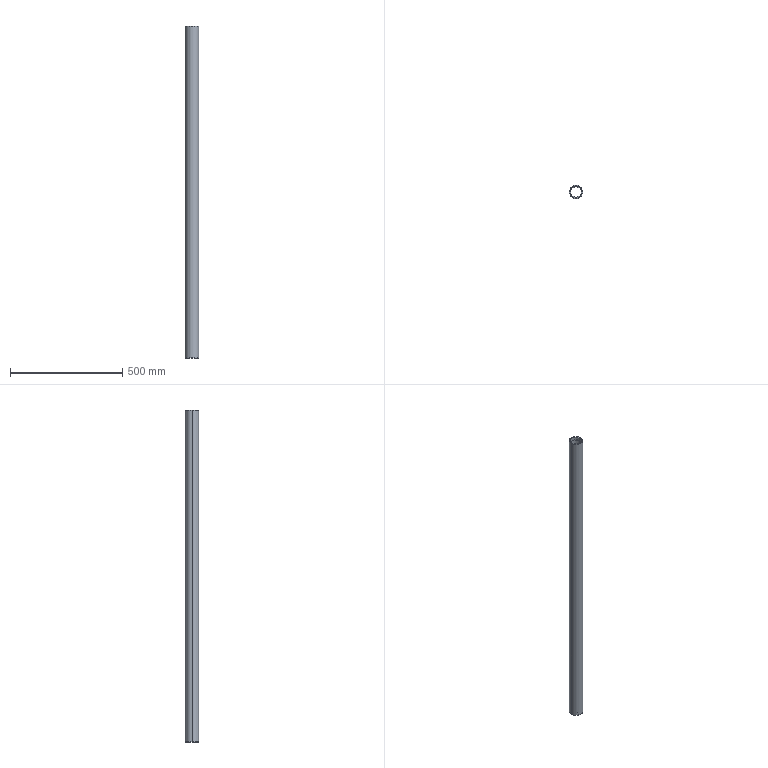Part | SolidWorks | features ICE 3, Chamfer 1, Extrusion 1 | 1 solid | 20 faces | box 60 x 60 x 1480 mm | volume 1496944 mm3 | cone 8 | cylinder 8 | plane 4 | commonest cylinder face diameters 52 x4 48 x2 60 x2
STEP:
#1=CARTESIAN_POINT('',(29.5,0.,1480.));
#2=VERTEX_POINT('',#1);
#3=CARTESIAN_POINT('',(-29.5,0.,1480.));
#4=VERTEX_POINT('',#3);
#5=CARTESIAN_POINT('',(0.,0.,1480.));
#6=DIRECTION('',(0.,0.,1.));
#7=DIRECTION('',(1.,0.,0.));
#8=AXIS2_PLACEMENT_3D('',#5,#6,#7);
#9=CIRCLE('',#8,29.5);
#10=EDGE_CURVE('',#2,#4,#9,.T.);
#11=ORIENTED_EDGE('',*,*,#10,.F.);
#12=CARTESIAN_POINT('',(30.,0.,1479.5));
#13=VERTEX_POINT('',#12);
#14=CARTESIAN_POINT('',(29.5,0.,1480.));
#15=DIRECTION('',(0.7071,0.,-0.7071));
#16=VECTOR('',#15,1000.);
#17=LINE('',#14,#16);
#18=EDGE_CURVE('',#2,#13,#17,.T.);
#19=ORIENTED_EDGE('',*,*,#18,.T.);
#20=CARTESIAN_POINT('',(-30.,0.,1479.5));
#21=VERTEX_POINT('',#20);
#22=CARTESIAN_POINT('',(0.,0.,1479.5));
#23=DIRECTION('',(0.,0.,-1.));
#24=DIRECTION('',(1.,0.,0.));
#25=AXIS2_PLACEMENT_3D('',#22,#23,#24);
#26=CIRCLE('',#25,30.);
#27=EDGE_CURVE('',#21,#13,#26,.T.);
#28=ORIENTED_EDGE('',*,*,#27,.F.);
#29=CARTESIAN_POINT('',(-29.5,0.,1480.));
#30=DIRECTION('',(-0.7071,0.,-0.7071));
#31=VECTOR('',#30,1000.);
#32=LINE('',#29,#31);
#33=EDGE_CURVE('',#4,#21,#32,.T.);
#34=ORIENTED_EDGE('',*,*,#33,.F.);
#35=EDGE_LOOP('',(#11,#19,#28,#34));
#36=FACE_OUTER_BOUND('',#35,.T.);
#37=CARTESIAN_POINT('',(0.,0.,1480.));
#38=DIRECTION('',(0.,0.,-1.));
#39=DIRECTION('',(-1.,0.,0.));
#40=AXIS2_PLACEMENT_3D('',#37,#38,#39);
#41=CONICAL_SURFACE('',#40,29.5,0.7854);
#42=ADVANCED_FACE('',(#36),#41,.T.);
#43=CARTESIAN_POINT('',(-26.,0.,1479.5));
#44=VERTEX_POINT('',#43);
#45=CARTESIAN_POINT('',(26.,0.,1479.5));
#46=VERTEX_POINT('',#45);
#47=CARTESIAN_POINT('',(0.,0.,1479.5));
#48=DIRECTION('',(0.,0.,1.));
#49=DIRECTION('',(1.,0.,0.));
#50=AXIS2_PLACEMENT_3D('',#47,#48,#49);
#51=CIRCLE('',#50,26.);
#52=EDGE_CURVE('',#44,#46,#51,.T.);
#53=ORIENTED_EDGE('',*,*,#52,.F.);
#54=CARTESIAN_POINT('',(-26.5,0.,1480.));
#55=VERTEX_POINT('',#54);
#56=CARTESIAN_POINT('',(-26.,0.,1479.5));
#57=DIRECTION('',(-0.7071,0.,0.7071));
#58=VECTOR('',#57,1000.);
#59=LINE('',#56,#58);
#60=EDGE_CURVE('',#44,#55,#59,.T.);
#61=ORIENTED_EDGE('',*,*,#60,.T.);
#62=CARTESIAN_POINT('',(26.5,0.,1480.));
#63=VERTEX_POINT('',#62);
#64=CARTESIAN_POINT('',(0.,0.,1480.));
#65=DIRECTION('',(0.,0.,-1.));
#66=DIRECTION('',(1.,0.,0.));
#67=AXIS2_PLACEMENT_3D('',#64,#65,#66);
#68=CIRCLE('',#67,26.5);
#69=EDGE_CURVE('',#63,#55,#68,.T.);
#70=ORIENTED_EDGE('',*,*,#69,.F.);
#71=CARTESIAN_POINT('',(26.,0.,1479.5));
#72=DIRECTION('',(0.7071,0.,0.7071));
#73=VECTOR('',#72,1000.);
#74=LINE('',#71,#73);
#75=EDGE_CURVE('',#46,#63,#74,.T.);
#76=ORIENTED_EDGE('',*,*,#75,.F.);
#77=EDGE_LOOP('',(#53,#61,#70,#76));
#78=FACE_OUTER_BOUND('',#77,.T.);
#79=CARTESIAN_POINT('',(0.,0.,1479.5));
#80=DIRECTION('',(0.,0.,1.));
#81=DIRECTION('',(1.,0.,0.));
#82=AXIS2_PLACEMENT_3D('',#79,#80,#81);
#83=CONICAL_SURFACE('',#82,26.,0.7854);
#84=ADVANCED_FACE('',(#78),#83,.F.);
#85=CARTESIAN_POINT('',(-29.5,0.,0.));
#86=VERTEX_POINT('',#85);
#87=CARTESIAN_POINT('',(29.5,0.,0.));
#88=VERTEX_POINT('',#87);
#89=CARTESIAN_POINT('',(0.,0.,0.));
#90=DIRECTION('',(0.,0.,-1.));
#91=DIRECTION('',(1.,0.,0.));
#92=AXIS2_PLACEMENT_3D('',#89,#90,#91);
#93=CIRCLE('',#92,29.5);
#94=EDGE_CURVE('',#86,#88,#93,.T.);
#95=ORIENTED_EDGE('',*,*,#94,.F.);
#96=CARTESIAN_POINT('',(-30.,0.,0.5));
#97=VERTEX_POINT('',#96);
#98=CARTESIAN_POINT('',(-30.,0.,0.5));
#99=DIRECTION('',(-0.7071,0.,0.7071));
#100=VECTOR('',#99,1000.);
#101=LINE('',#98,#100);
#102=EDGE_CURVE('',#86,#97,#101,.T.);
#103=ORIENTED_EDGE('',*,*,#102,.T.);
#104=CARTESIAN_POINT('',(30.,0.,0.5));
#105=VERTEX_POINT('',#104);
#106=CARTESIAN_POINT('',(0.,0.,0.5));
#107=DIRECTION('',(0.,0.,1.));
#108=DIRECTION('',(1.,0.,0.));
#109=AXIS2_PLACEMENT_3D('',#106,#107,#108);
#110=CIRCLE('',#109,30.);
#111=EDGE_CURVE('',#105,#97,#110,.T.);
#112=ORIENTED_EDGE('',*,*,#111,.F.);
#113=CARTESIAN_POINT('',(30.,0.,0.5));
#114=DIRECTION('',(0.7071,0.,0.7071));
#115=VECTOR('',#114,1000.);
#116=LINE('',#113,#115);
#117=EDGE_CURVE('',#88,#105,#116,.T.);
#118=ORIENTED_EDGE('',*,*,#117,.F.);
#119=EDGE_LOOP('',(#95,#103,#112,#118));
#120=FACE_OUTER_BOUND('',#119,.T.);
#121=CARTESIAN_POINT('',(0.,0.,0.5));
#122=DIRECTION('',(0.,0.,1.));
#123=DIRECTION('',(1.,0.,0.));
#124=AXIS2_PLACEMENT_3D('',#121,#122,#123);
#125=CONICAL_SURFACE('',#124,30.,0.7854);
#126=ADVANCED_FACE('',(#120),#125,.T.);
#127=CARTESIAN_POINT('',(26.,0.,0.5));
#128=VERTEX_POINT('',#127);
#129=CARTESIAN_POINT('',(-26.,0.,0.5));
#130=VERTEX_POINT('',#129);
#131=CARTESIAN_POINT('',(0.,0.,0.5));
#132=DIRECTION('',(0.,0.,-1.));
#133=DIRECTION('',(1.,0.,0.));
#134=AXIS2_PLACEMENT_3D('',#131,#132,#133);
#135=CIRCLE('',#134,26.);
#136=EDGE_CURVE('',#128,#130,#135,.T.);
#137=ORIENTED_EDGE('',*,*,#136,.F.);
#138=CARTESIAN_POINT('',(26.5,0.,0.));
#139=VERTEX_POINT('',#138);
#140=CARTESIAN_POINT('',(26.,0.,0.5));
#141=DIRECTION('',(0.7071,0.,-0.7071));
#142=VECTOR('',#141,1000.);
#143=LINE('',#140,#142);
#144=EDGE_CURVE('',#128,#139,#143,.T.);
#145=ORIENTED_EDGE('',*,*,#144,.T.);
#146=CARTESIAN_POINT('',(-26.5,0.,0.));
#147=VERTEX_POINT('',#146);
#148=CARTESIAN_POINT('',(0.,0.,0.));
#149=DIRECTION('',(0.,0.,1.));
#150=DIRECTION('',(1.,0.,0.));
#151=AXIS2_PLACEMENT_3D('',#148,#149,#150);
#152=CIRCLE('',#151,26.5);
#153=EDGE_CURVE('',#147,#139,#152,.T.);
#154=ORIENTED_EDGE('',*,*,#153,.F.);
#155=CARTESIAN_POINT('',(-26.,0.,0.5));
#156=DIRECTION('',(-0.7071,0.,-0.7071));
#157=VECTOR('',#156,1000.);
#158=LINE('',#155,#157);
#159=EDGE_CURVE('',#130,#147,#158,.T.);
#160=ORIENTED_EDGE('',*,*,#159,.F.);
#161=EDGE_LOOP('',(#137,#145,#154,#160));
#162=FACE_OUTER_BOUND('',#161,.T.);
#163=CARTESIAN_POINT('',(0.,0.,0.5));
#164=DIRECTION('',(0.,0.,-1.));
#165=DIRECTION('',(-1.,0.,0.));
#166=AXIS2_PLACEMENT_3D('',#163,#164,#165);
#167=CONICAL_SURFACE('',#166,26.,0.7854);
#168=ADVANCED_FACE('',(#162),#167,.F.);
#169=CARTESIAN_POINT('',(-26.,0.,1465.));
#170=VERTEX_POINT('',#169);
#171=CARTESIAN_POINT('',(26.,0.,1465.));
#172=VERTEX_POINT('',#171);
#173=CARTESIAN_POINT('',(0.,0.,1465.));
#174=DIRECTION('',(0.,0.,1.));
#175=DIRECTION('',(1.,0.,0.));
#176=AXIS2_PLACEMENT_3D('',#173,#174,#175);
#177=CIRCLE('',#176,26.);
#178=EDGE_CURVE('',#170,#172,#177,.T.);
#179=ORIENTED_EDGE('',*,*,#178,.F.);
#180=CARTESIAN_POINT('',(-26.,0.,1465.));
#181=DIRECTION('',(0.,0.,1.));
#182=VECTOR('',#181,1000.);
#183=LINE('',#180,#182);
#184=EDGE_CURVE('',#170,#44,#183,.T.);
#185=ORIENTED_EDGE('',*,*,#184,.T.);
#186=ORIENTED_EDGE('',*,*,#52,.T.);
#187=CARTESIAN_POINT('',(26.,0.,1465.));
#188=DIRECTION('',(0.,0.,1.));
#189=VECTOR('',#188,1000.);
#190=LINE('',#187,#189);
#191=EDGE_CURVE('',#172,#46,#190,.T.);
#192=ORIENTED_EDGE('',*,*,#191,.F.);
#193=EDGE_LOOP('',(#179,#185,#186,#192));
#194=FACE_OUTER_BOUND('',#193,.T.);
#195=CARTESIAN_POINT('',(0.,0.,1465.));
#196=DIRECTION('',(0.,0.,1.));
#197=DIRECTION('',(1.,0.,0.));
#198=AXIS2_PLACEMENT_3D('',#195,#196,#197);
#199=CYLINDRICAL_SURFACE('',#198,26.);
#200=ADVANCED_FACE('',(#194),#199,.F.);
#201=CARTESIAN_POINT('',(26.,0.,15.));
#202=VERTEX_POINT('',#201);
#203=CARTESIAN_POINT('',(-26.,0.,15.));
#204=VERTEX_POINT('',#203);
#205=CARTESIAN_POINT('',(0.,0.,15.));
#206=DIRECTION('',(0.,0.,-1.));
#207=DIRECTION('',(-1.,0.,0.));
#208=AXIS2_PLACEMENT_3D('',#205,#206,#207);
#209=CIRCLE('',#208,26.);
#210=EDGE_CURVE('',#202,#204,#209,.T.);
#211=ORIENTED_EDGE('',*,*,#210,.F.);
#212=CARTESIAN_POINT('',(26.,0.,15.));
#213=DIRECTION('',(0.,0.,-1.));
#214=VECTOR('',#213,1000.);
#215=LINE('',#212,#214);
#216=EDGE_CURVE('',#202,#128,#215,.T.);
#217=ORIENTED_EDGE('',*,*,#216,.T.);
#218=ORIENTED_EDGE('',*,*,#136,.T.);
#219=CARTESIAN_POINT('',(-26.,0.,15.));
#220=DIRECTION('',(0.,0.,-1.));
#221=VECTOR('',#220,1000.);
#222=LINE('',#219,#221);
#223=EDGE_CURVE('',#204,#130,#222,.T.);
#224=ORIENTED_EDGE('',*,*,#223,.F.);
#225=EDGE_LOOP('',(#211,#217,#218,#224));
#226=FACE_OUTER_BOUND('',#225,.T.);
#227=CARTESIAN_POINT('',(0.,0.,15.));
#228=DIRECTION('',(0.,0.,-1.));
#229=DIRECTION('',(-1.,0.,0.));
#230=AXIS2_PLACEMENT_3D('',#227,#228,#229);
#231=CYLINDRICAL_SURFACE('',#230,26.);
#232=ADVANCED_FACE('',(#226),#231,.F.);
#233=ORIENTED_EDGE('',*,*,#27,.T.);
#234=CARTESIAN_POINT('',(30.,0.,1480.));
#235=DIRECTION('',(0.,0.,-1.));
#236=VECTOR('',#235,1000.);
#237=LINE('',#234,#236);
#238=EDGE_CURVE('',#13,#105,#237,.T.);
#239=ORIENTED_EDGE('',*,*,#238,.T.);
#240=ORIENTED_EDGE('',*,*,#111,.T.);
#241=CARTESIAN_POINT('',(-30.,0.,1480.));
#242=DIRECTION('',(0.,0.,-1.));
#243=VECTOR('',#242,1000.);
#244=LINE('',#241,#243);
#245=EDGE_CURVE('',#21,#97,#244,.T.);
#246=ORIENTED_EDGE('',*,*,#245,.F.);
#247=EDGE_LOOP('',(#233,#239,#240,#246));
#248=FACE_OUTER_BOUND('',#247,.T.);
#249=CARTESIAN_POINT('',(0.,0.,1480.));
#250=DIRECTION('',(0.,0.,-1.));
#251=DIRECTION('',(-1.,0.,0.));
#252=AXIS2_PLACEMENT_3D('',#249,#250,#251);
#253=CYLINDRICAL_SURFACE('',#252,30.);
#254=ADVANCED_FACE('',(#248),#253,.T.);
#255=CARTESIAN_POINT('',(24.,0.,1465.));
#256=VERTEX_POINT('',#255);
#257=CARTESIAN_POINT('',(-24.,0.,1465.));
#258=VERTEX_POINT('',#257);
#259=CARTESIAN_POINT('',(0.,0.,1465.));
#260=DIRECTION('',(0.,0.,-1.));
#261=DIRECTION('',(1.,0.,0.));
#262=AXIS2_PLACEMENT_3D('',#259,#260,#261);
#263=CIRCLE('',#262,24.);
#264=EDGE_CURVE('',#256,#258,#263,.T.);
#265=ORIENTED_EDGE('',*,*,#264,.F.);
#266=CARTESIAN_POINT('',(24.,0.,15.));
#267=VERTEX_POINT('',#266);
#268=CARTESIAN_POINT('',(24.,0.,1600.));
#269=DIRECTION('',(0.,0.,-1.));
#270=VECTOR('',#269,1000.);
#271=LINE('',#268,#270);
#272=EDGE_CURVE('',#256,#267,#271,.T.);
#273=ORIENTED_EDGE('',*,*,#272,.T.);
#274=CARTESIAN_POINT('',(-24.,0.,15.));
#275=VERTEX_POINT('',#274);
#276=CARTESIAN_POINT('',(0.,0.,15.));
#277=DIRECTION('',(0.,0.,1.));
#278=DIRECTION('',(-1.,0.,0.));
#279=AXIS2_PLACEMENT_3D('',#276,#277,#278);
#280=CIRCLE('',#279,24.);
#281=EDGE_CURVE('',#275,#267,#280,.T.);
#282=ORIENTED_EDGE('',*,*,#281,.F.);
#283=CARTESIAN_POINT('',(-24.,0.,1600.));
#284=DIRECTION('',(0.,0.,-1.));
#285=VECTOR('',#284,1000.);
#286=LINE('',#283,#285);
#287=EDGE_CURVE('',#258,#275,#286,.T.);
#288=ORIENTED_EDGE('',*,*,#287,.F.);
#289=EDGE_LOOP('',(#265,#273,#282,#288));
#290=FACE_OUTER_BOUND('',#289,.T.);
#291=CARTESIAN_POINT('',(0.,0.,1600.));
#292=DIRECTION('',(0.,0.,-1.));
#293=DIRECTION('',(-1.,0.,0.));
#294=AXIS2_PLACEMENT_3D('',#291,#292,#293);
#295=CYLINDRICAL_SURFACE('',#294,24.);
#296=ADVANCED_FACE('',(#290),#295,.F.);
#297=ORIENTED_EDGE('',*,*,#272,.F.);
#298=CARTESIAN_POINT('',(0.,0.,1465.));
#299=DIRECTION('',(0.,0.,-1.));
#300=DIRECTION('',(1.,0.,0.));
#301=AXIS2_PLACEMENT_3D('',#298,#299,#300);
#302=CIRCLE('',#301,24.);
#303=EDGE_CURVE('',#258,#256,#302,.T.);
#304=ORIENTED_EDGE('',*,*,#303,.F.);
#305=ORIENTED_EDGE('',*,*,#287,.T.);
#306=CARTESIAN_POINT('',(0.,0.,15.));
#307=DIRECTION('',(0.,0.,1.));
#308=DIRECTION('',(-1.,0.,0.));
#309=AXIS2_PLACEMENT_3D('',#306,#307,#308);
#310=CIRCLE('',#309,24.);
#311=EDGE_CURVE('',#267,#275,#310,.T.);
#312=ORIENTED_EDGE('',*,*,#311,.F.);
#313=EDGE_LOOP('',(#297,#304,#305,#312));
#314=FACE_OUTER_BOUND('',#313,.T.);
#315=CARTESIAN_POINT('',(0.,0.,1600.));
#316=DIRECTION('',(0.,0.,-1.));
#317=DIRECTION('',(-1.,0.,0.));
#318=AXIS2_PLACEMENT_3D('',#315,#316,#317);
#319=CYLINDRICAL_SURFACE('',#318,24.);
#320=ADVANCED_FACE('',(#314),#319,.F.);
#321=ORIENTED_EDGE('',*,*,#238,.F.);
#322=CARTESIAN_POINT('',(0.,0.,1479.5));
#323=DIRECTION('',(0.,0.,-1.));
#324=DIRECTION('',(1.,0.,0.));
#325=AXIS2_PLACEMENT_3D('',#322,#323,#324);
#326=CIRCLE('',#325,30.);
#327=EDGE_CURVE('',#13,#21,#326,.T.);
#328=ORIENTED_EDGE('',*,*,#327,.T.);
#329=ORIENTED_EDGE('',*,*,#245,.T.);
#330=CARTESIAN_POINT('',(0.,0.,0.5));
#331=DIRECTION('',(0.,0.,1.));
#332=DIRECTION('',(1.,0.,0.));
#333=AXIS2_PLACEMENT_3D('',#330,#331,#332);
#334=CIRCLE('',#333,30.);
#335=EDGE_CURVE('',#97,#105,#334,.T.);
#336=ORIENTED_EDGE('',*,*,#335,.T.);
#337=EDGE_LOOP('',(#321,#328,#329,#336));
#338=FACE_OUTER_BOUND('',#337,.T.);
#339=CARTESIAN_POINT('',(0.,0.,1480.));
#340=DIRECTION('',(0.,0.,-1.));
#341=DIRECTION('',(-1.,0.,0.));
#342=AXIS2_PLACEMENT_3D('',#339,#340,#341);
#343=CYLINDRICAL_SURFACE('',#342,30.);
#344=ADVANCED_FACE('',(#338),#343,.T.);
#345=ORIENTED_EDGE('',*,*,#69,.T.);
#346=CARTESIAN_POINT('',(0.,0.,1480.));
#347=DIRECTION('',(0.,0.,-1.));
#348=DIRECTION('',(1.,0.,0.));
#349=AXIS2_PLACEMENT_3D('',#346,#347,#348);
#350=CIRCLE('',#349,26.5);
#351=EDGE_CURVE('',#55,#63,#350,.T.);
#352=ORIENTED_EDGE('',*,*,#351,.T.);
#353=EDGE_LOOP('',(#345,#352));
#354=FACE_BOUND('',#353,.T.);
#355=CARTESIAN_POINT('',(0.,0.,1480.));
#356=DIRECTION('',(0.,0.,1.));
#357=DIRECTION('',(1.,0.,0.));
#358=AXIS2_PLACEMENT_3D('',#355,#356,#357);
#359=CIRCLE('',#358,29.5);
#360=EDGE_CURVE('',#4,#2,#359,.T.);
#361=ORIENTED_EDGE('',*,*,#360,.T.);
#362=ORIENTED_EDGE('',*,*,#10,.T.);
#363=EDGE_LOOP('',(#361,#362));
#364=FACE_OUTER_BOUND('',#363,.T.);
#365=CARTESIAN_POINT('',(0.,0.,1480.));
#366=DIRECTION('',(0.,0.,1.));
#367=DIRECTION('',(1.,0.,0.));
#368=AXIS2_PLACEMENT_3D('',#365,#366,#367);
#369=PLANE('',#368);
#370=ADVANCED_FACE('',(#354,#364),#369,.T.);
#371=ORIENTED_EDGE('',*,*,#153,.T.);
#372=CARTESIAN_POINT('',(0.,0.,0.));
#373=DIRECTION('',(0.,0.,1.));
#374=DIRECTION('',(1.,0.,0.));
#375=AXIS2_PLACEMENT_3D('',#372,#373,#374);
#376=CIRCLE('',#375,26.5);
#377=EDGE_CURVE('',#139,#147,#376,.T.);
#378=ORIENTED_EDGE('',*,*,#377,.T.);
#379=EDGE_LOOP('',(#371,#378));
#380=FACE_BOUND('',#379,.T.);
#381=CARTESIAN_POINT('',(0.,0.,0.));
#382=DIRECTION('',(0.,0.,-1.));
#383=DIRECTION('',(1.,0.,0.));
#384=AXIS2_PLACEMENT_3D('',#381,#382,#383);
#385=CIRCLE('',#384,29.5);
#386=EDGE_CURVE('',#88,#86,#385,.T.);
#387=ORIENTED_EDGE('',*,*,#386,.T.);
#388=ORIENTED_EDGE('',*,*,#94,.T.);
#389=EDGE_LOOP('',(#387,#388));
#390=FACE_OUTER_BOUND('',#389,.T.);
#391=CARTESIAN_POINT('',(0.,0.,0.));
#392=DIRECTION('',(0.,0.,1.));
#393=DIRECTION('',(1.,0.,0.));
#394=AXIS2_PLACEMENT_3D('',#391,#392,#393);
#395=PLANE('',#394);
#396=ADVANCED_FACE('',(#380,#390),#395,.F.);
#397=CARTESIAN_POINT('',(0.,0.,15.));
#398=DIRECTION('',(0.,0.,-1.));
#399=DIRECTION('',(-1.,0.,0.));
#400=AXIS2_PLACEMENT_3D('',#397,#398,#399);
#401=CIRCLE('',#400,26.);
#402=EDGE_CURVE('',#204,#202,#401,.T.);
#403=ORIENTED_EDGE('',*,*,#402,.T.);
#404=ORIENTED_EDGE('',*,*,#210,.T.);
#405=EDGE_LOOP('',(#403,#404));
#406=FACE_OUTER_BOUND('',#405,.T.);
#407=ORIENTED_EDGE('',*,*,#281,.T.);
#408=ORIENTED_EDGE('',*,*,#311,.T.);
#409=EDGE_LOOP('',(#407,#408));
#410=FACE_BOUND('',#409,.T.);
#411=CARTESIAN_POINT('',(0.,0.,15.));
#412=DIRECTION('',(0.,0.,-1.));
#413=DIRECTION('',(-1.,0.,0.));
#414=AXIS2_PLACEMENT_3D('',#411,#412,#413);
#415=PLANE('',#414);
#416=ADVANCED_FACE('',(#406,#410),#415,.T.);
#417=ORIENTED_EDGE('',*,*,#216,.F.);
#418=ORIENTED_EDGE('',*,*,#402,.F.);
#419=ORIENTED_EDGE('',*,*,#223,.T.);
#420=CARTESIAN_POINT('',(0.,0.,0.5));
#421=DIRECTION('',(0.,0.,-1.));
#422=DIRECTION('',(1.,0.,0.));
#423=AXIS2_PLACEMENT_3D('',#420,#421,#422);
#424=CIRCLE('',#423,26.);
#425=EDGE_CURVE('',#130,#128,#424,.T.);
#426=ORIENTED_EDGE('',*,*,#425,.T.);
#427=EDGE_LOOP('',(#417,#418,#419,#426));
#428=FACE_OUTER_BOUND('',#427,.T.);
#429=CARTESIAN_POINT('',(0.,0.,15.));
#430=DIRECTION('',(0.,0.,-1.));
#431=DIRECTION('',(-1.,0.,0.));
#432=AXIS2_PLACEMENT_3D('',#429,#430,#431);
#433=CYLINDRICAL_SURFACE('',#432,26.);
#434=ADVANCED_FACE('',(#428),#433,.F.);
#435=CARTESIAN_POINT('',(0.,0.,1465.));
#436=DIRECTION('',(0.,0.,1.));
#437=DIRECTION('',(1.,0.,0.));
#438=AXIS2_PLACEMENT_3D('',#435,#436,#437);
#439=CIRCLE('',#438,26.);
#440=EDGE_CURVE('',#172,#170,#439,.T.);
#441=ORIENTED_EDGE('',*,*,#440,.T.);
#442=ORIENTED_EDGE('',*,*,#178,.T.);
#443=EDGE_LOOP('',(#441,#442));
#444=FACE_OUTER_BOUND('',#443,.T.);
#445=ORIENTED_EDGE('',*,*,#303,.T.);
#446=ORIENTED_EDGE('',*,*,#264,.T.);
#447=EDGE_LOOP('',(#445,#446));
#448=FACE_BOUND('',#447,.T.);
#449=CARTESIAN_POINT('',(0.,0.,1465.));
#450=DIRECTION('',(0.,0.,1.));
#451=DIRECTION('',(1.,0.,0.));
#452=AXIS2_PLACEMENT_3D('',#449,#450,#451);
#453=PLANE('',#452);
#454=ADVANCED_FACE('',(#444,#448),#453,.T.);
#455=ORIENTED_EDGE('',*,*,#184,.F.);
#456=ORIENTED_EDGE('',*,*,#440,.F.);
#457=ORIENTED_EDGE('',*,*,#191,.T.);
#458=CARTESIAN_POINT('',(0.,0.,1479.5));
#459=DIRECTION('',(0.,0.,1.));
#460=DIRECTION('',(1.,0.,0.));
#461=AXIS2_PLACEMENT_3D('',#458,#459,#460);
#462=CIRCLE('',#461,26.);
#463=EDGE_CURVE('',#46,#44,#462,.T.);
#464=ORIENTED_EDGE('',*,*,#463,.T.);
#465=EDGE_LOOP('',(#455,#456,#457,#464));
#466=FACE_OUTER_BOUND('',#465,.T.);
#467=CARTESIAN_POINT('',(0.,0.,1465.));
#468=DIRECTION('',(0.,0.,1.));
#469=DIRECTION('',(1.,0.,0.));
#470=AXIS2_PLACEMENT_3D('',#467,#468,#469);
#471=CYLINDRICAL_SURFACE('',#470,26.);
#472=ADVANCED_FACE('',(#466),#471,.F.);
#473=ORIENTED_EDGE('',*,*,#144,.F.);
#474=ORIENTED_EDGE('',*,*,#425,.F.);
#475=ORIENTED_EDGE('',*,*,#159,.T.);
#476=ORIENTED_EDGE('',*,*,#377,.F.);
#477=EDGE_LOOP('',(#473,#474,#475,#476));
#478=FACE_OUTER_BOUND('',#477,.T.);
#479=CARTESIAN_POINT('',(0.,0.,0.5));
#480=DIRECTION('',(0.,0.,-1.));
#481=DIRECTION('',(-1.,0.,0.));
#482=AXIS2_PLACEMENT_3D('',#479,#480,#481);
#483=CONICAL_SURFACE('',#482,26.,0.7854);
#484=ADVANCED_FACE('',(#478),#483,.F.);
#485=ORIENTED_EDGE('',*,*,#102,.F.);
#486=ORIENTED_EDGE('',*,*,#386,.F.);
#487=ORIENTED_EDGE('',*,*,#117,.T.);
#488=ORIENTED_EDGE('',*,*,#335,.F.);
#489=EDGE_LOOP('',(#485,#486,#487,#488));
#490=FACE_OUTER_BOUND('',#489,.T.);
#491=CARTESIAN_POINT('',(0.,0.,0.5));
#492=DIRECTION('',(0.,0.,1.));
#493=DIRECTION('',(1.,0.,0.));
#494=AXIS2_PLACEMENT_3D('',#491,#492,#493);
#495=CONICAL_SURFACE('',#494,30.,0.7854);
#496=ADVANCED_FACE('',(#490),#495,.T.);
#497=ORIENTED_EDGE('',*,*,#60,.F.);
#498=ORIENTED_EDGE('',*,*,#463,.F.);
#499=ORIENTED_EDGE('',*,*,#75,.T.);
#500=ORIENTED_EDGE('',*,*,#351,.F.);
#501=EDGE_LOOP('',(#497,#498,#499,#500));
#502=FACE_OUTER_BOUND('',#501,.T.);
#503=CARTESIAN_POINT('',(0.,0.,1479.5));
#504=DIRECTION('',(0.,0.,1.));
#505=DIRECTION('',(1.,0.,0.));
#506=AXIS2_PLACEMENT_3D('',#503,#504,#505);
#507=CONICAL_SURFACE('',#506,26.,0.7854);
#508=ADVANCED_FACE('',(#502),#507,.F.);
#509=ORIENTED_EDGE('',*,*,#18,.F.);
#510=ORIENTED_EDGE('',*,*,#360,.F.);
#511=ORIENTED_EDGE('',*,*,#33,.T.);
#512=ORIENTED_EDGE('',*,*,#327,.F.);
#513=EDGE_LOOP('',(#509,#510,#511,#512));
#514=FACE_OUTER_BOUND('',#513,.T.);
#515=CARTESIAN_POINT('',(0.,0.,1480.));
#516=DIRECTION('',(0.,0.,-1.));
#517=DIRECTION('',(-1.,0.,0.));
#518=AXIS2_PLACEMENT_3D('',#515,#516,#517);
#519=CONICAL_SURFACE('',#518,29.5,0.7854);
#520=ADVANCED_FACE('',(#514),#519,.T.);
#521=CLOSED_SHELL('',(#42,#84,#126,#168,#200,#232,#254,#296,#320,#344,#370,#396,#416,#434,#454,#472,#484,#496,#508,#520));
#522=MANIFOLD_SOLID_BREP('',#521);
#523=CARTESIAN_POINT('',(0.,0.,0.));
#524=DIRECTION('',(0.,0.,1.));
#525=DIRECTION('',(1.,0.,0.));
#526=AXIS2_PLACEMENT_3D('',#523,#524,#525);
#527=(LENGTH_UNIT()NAMED_UNIT(*)SI_UNIT(.MILLI.,.METRE.));
#528=UNCERTAINTY_MEASURE_WITH_UNIT(LENGTH_MEASURE(0.00001),#527,'','');
#529=(NAMED_UNIT(*)PLANE_ANGLE_UNIT()SI_UNIT($,.RADIAN.));
#530=(NAMED_UNIT(*)SI_UNIT($,.STERADIAN.)SOLID_ANGLE_UNIT());
#531=(GEOMETRIC_REPRESENTATION_CONTEXT(3)GLOBAL_UNCERTAINTY_ASSIGNED_CONTEXT((#528))GLOBAL_UNIT_ASSIGNED_CONTEXT((#527,#529,#530))REPRESENTATION_CONTEXT('',''));
#532=ADVANCED_BREP_SHAPE_REPRESENTATION('',(#522,#526),#531);